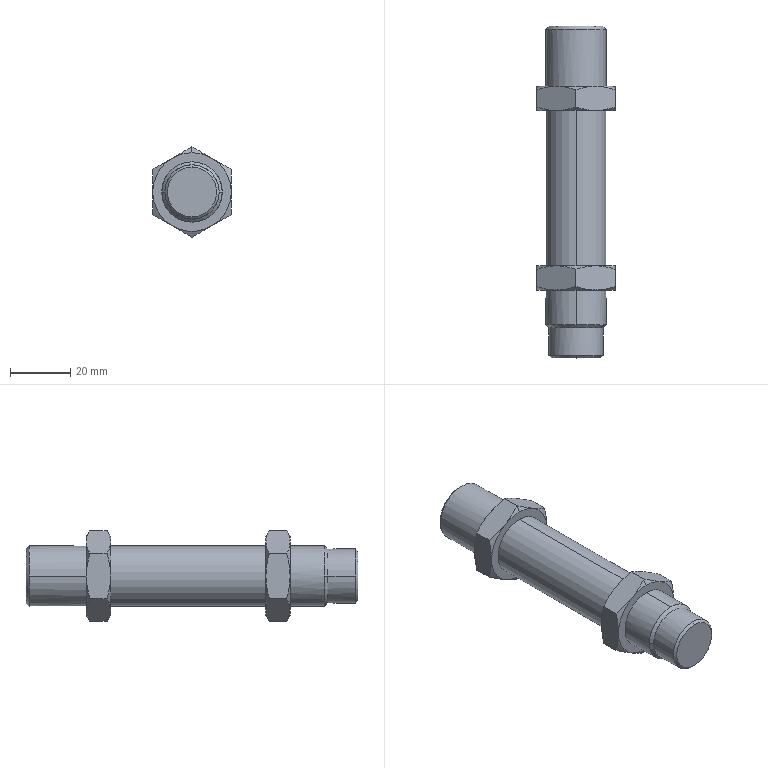Part | STEP file | 1 solid | 63 faces | box 26 x 110 x 30.022 mm | volume 37581 mm3 | cone 34 | plane 19 | cylinder 10 | commonest cylinder face diameters 20 x6 6 x2 18 x2